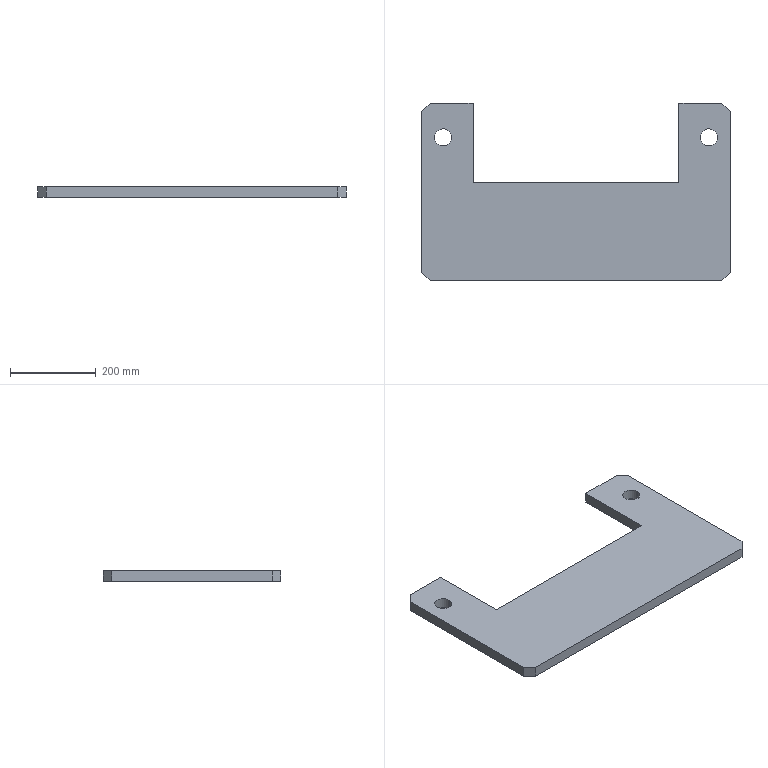Part | SolidWorks | features Chamfer 1, Extrusion 1 | 1 solid | 18 faces | box 720 x 415 x 25 mm | volume 5167168 mm3 | plane 14 | cylinder 4 | commonest cylinder face diameters 40 x4
STEP:
#1=CARTESIAN_POINT('',(650.,-80.,25.));
#2=VERTEX_POINT('',#1);
#3=CARTESIAN_POINT('',(690.,-80.,25.));
#4=VERTEX_POINT('',#3);
#5=CARTESIAN_POINT('',(670.,-80.,25.));
#6=DIRECTION('',(0.,0.,1.));
#7=DIRECTION('',(1.,0.,0.));
#8=AXIS2_PLACEMENT_3D('',#5,#6,#7);
#9=CIRCLE('',#8,20.);
#10=EDGE_CURVE('',#2,#4,#9,.T.);
#11=ORIENTED_EDGE('',*,*,#10,.T.);
#12=CARTESIAN_POINT('',(690.,-80.,0.));
#13=VERTEX_POINT('',#12);
#14=CARTESIAN_POINT('',(690.,-80.,25.));
#15=DIRECTION('',(0.,0.,-1.));
#16=VECTOR('',#15,1000.);
#17=LINE('',#14,#16);
#18=EDGE_CURVE('',#4,#13,#17,.T.);
#19=ORIENTED_EDGE('',*,*,#18,.T.);
#20=CARTESIAN_POINT('',(650.,-80.,0.));
#21=VERTEX_POINT('',#20);
#22=CARTESIAN_POINT('',(670.,-80.,0.));
#23=DIRECTION('',(0.,0.,1.));
#24=DIRECTION('',(1.,0.,0.));
#25=AXIS2_PLACEMENT_3D('',#22,#23,#24);
#26=CIRCLE('',#25,20.);
#27=EDGE_CURVE('',#21,#13,#26,.T.);
#28=ORIENTED_EDGE('',*,*,#27,.F.);
#29=CARTESIAN_POINT('',(650.,-80.,25.));
#30=DIRECTION('',(0.,0.,-1.));
#31=VECTOR('',#30,1000.);
#32=LINE('',#29,#31);
#33=EDGE_CURVE('',#2,#21,#32,.T.);
#34=ORIENTED_EDGE('',*,*,#33,.F.);
#35=EDGE_LOOP('',(#11,#19,#28,#34));
#36=FACE_OUTER_BOUND('',#35,.T.);
#37=CARTESIAN_POINT('',(670.,-80.,25.));
#38=DIRECTION('',(0.,0.,-1.));
#39=DIRECTION('',(-1.,0.,0.));
#40=AXIS2_PLACEMENT_3D('',#37,#38,#39);
#41=CYLINDRICAL_SURFACE('',#40,20.);
#42=ADVANCED_FACE('',(#36),#41,.F.);
#43=CARTESIAN_POINT('',(30.,-80.,25.));
#44=VERTEX_POINT('',#43);
#45=CARTESIAN_POINT('',(70.,-80.,25.));
#46=VERTEX_POINT('',#45);
#47=CARTESIAN_POINT('',(50.,-80.,25.));
#48=DIRECTION('',(0.,0.,1.));
#49=DIRECTION('',(1.,0.,0.));
#50=AXIS2_PLACEMENT_3D('',#47,#48,#49);
#51=CIRCLE('',#50,20.);
#52=EDGE_CURVE('',#44,#46,#51,.T.);
#53=ORIENTED_EDGE('',*,*,#52,.T.);
#54=CARTESIAN_POINT('',(70.,-80.,0.));
#55=VERTEX_POINT('',#54);
#56=CARTESIAN_POINT('',(70.,-80.,25.));
#57=DIRECTION('',(0.,0.,-1.));
#58=VECTOR('',#57,1000.);
#59=LINE('',#56,#58);
#60=EDGE_CURVE('',#46,#55,#59,.T.);
#61=ORIENTED_EDGE('',*,*,#60,.T.);
#62=CARTESIAN_POINT('',(30.,-80.,0.));
#63=VERTEX_POINT('',#62);
#64=CARTESIAN_POINT('',(50.,-80.,0.));
#65=DIRECTION('',(0.,0.,1.));
#66=DIRECTION('',(1.,0.,0.));
#67=AXIS2_PLACEMENT_3D('',#64,#65,#66);
#68=CIRCLE('',#67,20.);
#69=EDGE_CURVE('',#63,#55,#68,.T.);
#70=ORIENTED_EDGE('',*,*,#69,.F.);
#71=CARTESIAN_POINT('',(30.,-80.,25.));
#72=DIRECTION('',(0.,0.,-1.));
#73=VECTOR('',#72,1000.);
#74=LINE('',#71,#73);
#75=EDGE_CURVE('',#44,#63,#74,.T.);
#76=ORIENTED_EDGE('',*,*,#75,.F.);
#77=EDGE_LOOP('',(#53,#61,#70,#76));
#78=FACE_OUTER_BOUND('',#77,.T.);
#79=CARTESIAN_POINT('',(50.,-80.,25.));
#80=DIRECTION('',(0.,0.,-1.));
#81=DIRECTION('',(-1.,0.,0.));
#82=AXIS2_PLACEMENT_3D('',#79,#80,#81);
#83=CYLINDRICAL_SURFACE('',#82,20.);
#84=ADVANCED_FACE('',(#78),#83,.F.);
#85=CARTESIAN_POINT('',(600.,-185.,0.));
#86=VERTEX_POINT('',#85);
#87=CARTESIAN_POINT('',(120.,-185.,0.));
#88=VERTEX_POINT('',#87);
#89=CARTESIAN_POINT('',(0.,-185.,0.));
#90=DIRECTION('',(-1.,0.,0.));
#91=VECTOR('',#90,1000.);
#92=LINE('',#89,#91);
#93=EDGE_CURVE('',#86,#88,#92,.T.);
#94=ORIENTED_EDGE('',*,*,#93,.T.);
#95=CARTESIAN_POINT('',(120.,-185.,25.));
#96=VERTEX_POINT('',#95);
#97=CARTESIAN_POINT('',(120.,-185.,25.));
#98=DIRECTION('',(0.,0.,-1.));
#99=VECTOR('',#98,1000.);
#100=LINE('',#97,#99);
#101=EDGE_CURVE('',#96,#88,#100,.T.);
#102=ORIENTED_EDGE('',*,*,#101,.F.);
#103=CARTESIAN_POINT('',(600.,-185.,25.));
#104=VERTEX_POINT('',#103);
#105=CARTESIAN_POINT('',(0.,-185.,25.));
#106=DIRECTION('',(-1.,0.,0.));
#107=VECTOR('',#106,1000.);
#108=LINE('',#105,#107);
#109=EDGE_CURVE('',#104,#96,#108,.T.);
#110=ORIENTED_EDGE('',*,*,#109,.F.);
#111=CARTESIAN_POINT('',(600.,-185.,25.));
#112=DIRECTION('',(0.,0.,-1.));
#113=VECTOR('',#112,1000.);
#114=LINE('',#111,#113);
#115=EDGE_CURVE('',#104,#86,#114,.T.);
#116=ORIENTED_EDGE('',*,*,#115,.T.);
#117=EDGE_LOOP('',(#94,#102,#110,#116));
#118=FACE_OUTER_BOUND('',#117,.T.);
#119=CARTESIAN_POINT('',(0.,-185.,25.));
#120=DIRECTION('',(0.,-1.,0.));
#121=DIRECTION('',(1.,0.,0.));
#122=AXIS2_PLACEMENT_3D('',#119,#120,#121);
#123=PLANE('',#122);
#124=ADVANCED_FACE('',(#118),#123,.F.);
#125=CARTESIAN_POINT('',(120.,0.,0.));
#126=VERTEX_POINT('',#125);
#127=CARTESIAN_POINT('',(120.,0.,0.));
#128=DIRECTION('',(0.,1.,0.));
#129=VECTOR('',#128,1000.);
#130=LINE('',#127,#129);
#131=EDGE_CURVE('',#88,#126,#130,.T.);
#132=ORIENTED_EDGE('',*,*,#131,.T.);
#133=CARTESIAN_POINT('',(120.,0.,25.));
#134=VERTEX_POINT('',#133);
#135=CARTESIAN_POINT('',(120.,0.,25.));
#136=DIRECTION('',(0.,0.,-1.));
#137=VECTOR('',#136,1000.);
#138=LINE('',#135,#137);
#139=EDGE_CURVE('',#134,#126,#138,.T.);
#140=ORIENTED_EDGE('',*,*,#139,.F.);
#141=CARTESIAN_POINT('',(120.,0.,25.));
#142=DIRECTION('',(0.,1.,0.));
#143=VECTOR('',#142,1000.);
#144=LINE('',#141,#143);
#145=EDGE_CURVE('',#96,#134,#144,.T.);
#146=ORIENTED_EDGE('',*,*,#145,.F.);
#147=ORIENTED_EDGE('',*,*,#101,.T.);
#148=EDGE_LOOP('',(#132,#140,#146,#147));
#149=FACE_OUTER_BOUND('',#148,.T.);
#150=CARTESIAN_POINT('',(120.,0.,25.));
#151=DIRECTION('',(-1.,0.,0.));
#152=DIRECTION('',(0.,0.,1.));
#153=AXIS2_PLACEMENT_3D('',#150,#151,#152);
#154=PLANE('',#153);
#155=ADVANCED_FACE('',(#149),#154,.F.);
#156=CARTESIAN_POINT('',(20.,0.,0.));
#157=VERTEX_POINT('',#156);
#158=CARTESIAN_POINT('',(0.,0.,0.));
#159=DIRECTION('',(1.,0.,0.));
#160=VECTOR('',#159,1000.);
#161=LINE('',#158,#160);
#162=EDGE_CURVE('',#157,#126,#161,.T.);
#163=ORIENTED_EDGE('',*,*,#162,.F.);
#164=CARTESIAN_POINT('',(20.,0.,25.));
#165=VERTEX_POINT('',#164);
#166=CARTESIAN_POINT('',(20.,0.,25.));
#167=DIRECTION('',(0.,0.,1.));
#168=VECTOR('',#167,1000.);
#169=LINE('',#166,#168);
#170=EDGE_CURVE('',#157,#165,#169,.T.);
#171=ORIENTED_EDGE('',*,*,#170,.T.);
#172=CARTESIAN_POINT('',(0.,0.,25.));
#173=DIRECTION('',(1.,0.,0.));
#174=VECTOR('',#173,1000.);
#175=LINE('',#172,#174);
#176=EDGE_CURVE('',#165,#134,#175,.T.);
#177=ORIENTED_EDGE('',*,*,#176,.T.);
#178=ORIENTED_EDGE('',*,*,#139,.T.);
#179=EDGE_LOOP('',(#163,#171,#177,#178));
#180=FACE_OUTER_BOUND('',#179,.T.);
#181=CARTESIAN_POINT('',(0.,0.,25.));
#182=DIRECTION('',(0.,1.,0.));
#183=DIRECTION('',(0.,0.,1.));
#184=AXIS2_PLACEMENT_3D('',#181,#182,#183);
#185=PLANE('',#184);
#186=ADVANCED_FACE('',(#180),#185,.T.);
#187=CARTESIAN_POINT('',(0.,-20.,25.));
#188=VERTEX_POINT('',#187);
#189=CARTESIAN_POINT('',(0.,-395.,25.));
#190=VERTEX_POINT('',#189);
#191=CARTESIAN_POINT('',(0.,0.,25.));
#192=DIRECTION('',(0.,-1.,0.));
#193=VECTOR('',#192,1000.);
#194=LINE('',#191,#193);
#195=EDGE_CURVE('',#188,#190,#194,.T.);
#196=ORIENTED_EDGE('',*,*,#195,.F.);
#197=CARTESIAN_POINT('',(0.,-20.,0.));
#198=VERTEX_POINT('',#197);
#199=CARTESIAN_POINT('',(0.,-20.,0.));
#200=DIRECTION('',(0.,0.,-1.));
#201=VECTOR('',#200,1000.);
#202=LINE('',#199,#201);
#203=EDGE_CURVE('',#188,#198,#202,.T.);
#204=ORIENTED_EDGE('',*,*,#203,.T.);
#205=CARTESIAN_POINT('',(0.,-395.,0.));
#206=VERTEX_POINT('',#205);
#207=CARTESIAN_POINT('',(0.,0.,0.));
#208=DIRECTION('',(0.,-1.,0.));
#209=VECTOR('',#208,1000.);
#210=LINE('',#207,#209);
#211=EDGE_CURVE('',#198,#206,#210,.T.);
#212=ORIENTED_EDGE('',*,*,#211,.T.);
#213=CARTESIAN_POINT('',(0.,-395.,25.));
#214=DIRECTION('',(0.,0.,1.));
#215=VECTOR('',#214,1000.);
#216=LINE('',#213,#215);
#217=EDGE_CURVE('',#206,#190,#216,.T.);
#218=ORIENTED_EDGE('',*,*,#217,.T.);
#219=EDGE_LOOP('',(#196,#204,#212,#218));
#220=FACE_OUTER_BOUND('',#219,.T.);
#221=CARTESIAN_POINT('',(0.,0.,25.));
#222=DIRECTION('',(1.,0.,0.));
#223=DIRECTION('',(0.,1.,0.));
#224=AXIS2_PLACEMENT_3D('',#221,#222,#223);
#225=PLANE('',#224);
#226=ADVANCED_FACE('',(#220),#225,.F.);
#227=CARTESIAN_POINT('',(20.,-415.,25.));
#228=VERTEX_POINT('',#227);
#229=CARTESIAN_POINT('',(700.,-415.,25.));
#230=VERTEX_POINT('',#229);
#231=CARTESIAN_POINT('',(0.,-415.,25.));
#232=DIRECTION('',(1.,0.,0.));
#233=VECTOR('',#232,1000.);
#234=LINE('',#231,#233);
#235=EDGE_CURVE('',#228,#230,#234,.T.);
#236=ORIENTED_EDGE('',*,*,#235,.F.);
#237=CARTESIAN_POINT('',(20.,-415.,0.));
#238=VERTEX_POINT('',#237);
#239=CARTESIAN_POINT('',(20.,-415.,25.));
#240=DIRECTION('',(0.,0.,-1.));
#241=VECTOR('',#240,1000.);
#242=LINE('',#239,#241);
#243=EDGE_CURVE('',#228,#238,#242,.T.);
#244=ORIENTED_EDGE('',*,*,#243,.T.);
#245=CARTESIAN_POINT('',(700.,-415.,0.));
#246=VERTEX_POINT('',#245);
#247=CARTESIAN_POINT('',(0.,-415.,0.));
#248=DIRECTION('',(1.,0.,0.));
#249=VECTOR('',#248,1000.);
#250=LINE('',#247,#249);
#251=EDGE_CURVE('',#238,#246,#250,.T.);
#252=ORIENTED_EDGE('',*,*,#251,.T.);
#253=CARTESIAN_POINT('',(700.,-415.,25.));
#254=DIRECTION('',(0.,0.,1.));
#255=VECTOR('',#254,1000.);
#256=LINE('',#253,#255);
#257=EDGE_CURVE('',#246,#230,#256,.T.);
#258=ORIENTED_EDGE('',*,*,#257,.T.);
#259=EDGE_LOOP('',(#236,#244,#252,#258));
#260=FACE_OUTER_BOUND('',#259,.T.);
#261=CARTESIAN_POINT('',(0.,-415.,25.));
#262=DIRECTION('',(0.,1.,0.));
#263=DIRECTION('',(0.,0.,1.));
#264=AXIS2_PLACEMENT_3D('',#261,#262,#263);
#265=PLANE('',#264);
#266=ADVANCED_FACE('',(#260),#265,.F.);
#267=CARTESIAN_POINT('',(720.,-20.,25.));
#268=VERTEX_POINT('',#267);
#269=CARTESIAN_POINT('',(720.,-395.,25.));
#270=VERTEX_POINT('',#269);
#271=CARTESIAN_POINT('',(720.,0.,25.));
#272=DIRECTION('',(0.,-1.,0.));
#273=VECTOR('',#272,1000.);
#274=LINE('',#271,#273);
#275=EDGE_CURVE('',#268,#270,#274,.T.);
#276=ORIENTED_EDGE('',*,*,#275,.T.);
#277=CARTESIAN_POINT('',(720.,-395.,0.));
#278=VERTEX_POINT('',#277);
#279=CARTESIAN_POINT('',(720.,-395.,0.));
#280=DIRECTION('',(0.,0.,-1.));
#281=VECTOR('',#280,1000.);
#282=LINE('',#279,#281);
#283=EDGE_CURVE('',#270,#278,#282,.T.);
#284=ORIENTED_EDGE('',*,*,#283,.T.);
#285=CARTESIAN_POINT('',(720.,-20.,0.));
#286=VERTEX_POINT('',#285);
#287=CARTESIAN_POINT('',(720.,0.,0.));
#288=DIRECTION('',(0.,-1.,0.));
#289=VECTOR('',#288,1000.);
#290=LINE('',#287,#289);
#291=EDGE_CURVE('',#286,#278,#290,.T.);
#292=ORIENTED_EDGE('',*,*,#291,.F.);
#293=CARTESIAN_POINT('',(720.,-20.,25.));
#294=DIRECTION('',(0.,0.,1.));
#295=VECTOR('',#294,1000.);
#296=LINE('',#293,#295);
#297=EDGE_CURVE('',#286,#268,#296,.T.);
#298=ORIENTED_EDGE('',*,*,#297,.T.);
#299=EDGE_LOOP('',(#276,#284,#292,#298));
#300=FACE_OUTER_BOUND('',#299,.T.);
#301=CARTESIAN_POINT('',(720.,0.,25.));
#302=DIRECTION('',(1.,0.,0.));
#303=DIRECTION('',(0.,1.,0.));
#304=AXIS2_PLACEMENT_3D('',#301,#302,#303);
#305=PLANE('',#304);
#306=ADVANCED_FACE('',(#300),#305,.T.);
#307=CARTESIAN_POINT('',(600.,0.,25.));
#308=VERTEX_POINT('',#307);
#309=CARTESIAN_POINT('',(700.,0.,25.));
#310=VERTEX_POINT('',#309);
#311=CARTESIAN_POINT('',(0.,0.,25.));
#312=DIRECTION('',(1.,0.,0.));
#313=VECTOR('',#312,1000.);
#314=LINE('',#311,#313);
#315=EDGE_CURVE('',#308,#310,#314,.T.);
#316=ORIENTED_EDGE('',*,*,#315,.T.);
#317=CARTESIAN_POINT('',(700.,0.,0.));
#318=VERTEX_POINT('',#317);
#319=CARTESIAN_POINT('',(700.,0.,25.));
#320=DIRECTION('',(0.,0.,-1.));
#321=VECTOR('',#320,1000.);
#322=LINE('',#319,#321);
#323=EDGE_CURVE('',#310,#318,#322,.T.);
#324=ORIENTED_EDGE('',*,*,#323,.T.);
#325=CARTESIAN_POINT('',(600.,0.,0.));
#326=VERTEX_POINT('',#325);
#327=CARTESIAN_POINT('',(0.,0.,0.));
#328=DIRECTION('',(1.,0.,0.));
#329=VECTOR('',#328,1000.);
#330=LINE('',#327,#329);
#331=EDGE_CURVE('',#326,#318,#330,.T.);
#332=ORIENTED_EDGE('',*,*,#331,.F.);
#333=CARTESIAN_POINT('',(600.,0.,25.));
#334=DIRECTION('',(0.,0.,-1.));
#335=VECTOR('',#334,1000.);
#336=LINE('',#333,#335);
#337=EDGE_CURVE('',#308,#326,#336,.T.);
#338=ORIENTED_EDGE('',*,*,#337,.F.);
#339=EDGE_LOOP('',(#316,#324,#332,#338));
#340=FACE_OUTER_BOUND('',#339,.T.);
#341=CARTESIAN_POINT('',(0.,0.,25.));
#342=DIRECTION('',(0.,1.,0.));
#343=DIRECTION('',(0.,0.,1.));
#344=AXIS2_PLACEMENT_3D('',#341,#342,#343);
#345=PLANE('',#344);
#346=ADVANCED_FACE('',(#340),#345,.T.);
#347=ORIENTED_EDGE('',*,*,#60,.F.);
#348=CARTESIAN_POINT('',(50.,-80.,25.));
#349=DIRECTION('',(0.,0.,1.));
#350=DIRECTION('',(1.,0.,0.));
#351=AXIS2_PLACEMENT_3D('',#348,#349,#350);
#352=CIRCLE('',#351,20.);
#353=EDGE_CURVE('',#46,#44,#352,.T.);
#354=ORIENTED_EDGE('',*,*,#353,.T.);
#355=ORIENTED_EDGE('',*,*,#75,.T.);
#356=CARTESIAN_POINT('',(50.,-80.,0.));
#357=DIRECTION('',(0.,0.,1.));
#358=DIRECTION('',(1.,0.,0.));
#359=AXIS2_PLACEMENT_3D('',#356,#357,#358);
#360=CIRCLE('',#359,20.);
#361=EDGE_CURVE('',#55,#63,#360,.T.);
#362=ORIENTED_EDGE('',*,*,#361,.F.);
#363=EDGE_LOOP('',(#347,#354,#355,#362));
#364=FACE_OUTER_BOUND('',#363,.T.);
#365=CARTESIAN_POINT('',(50.,-80.,25.));
#366=DIRECTION('',(0.,0.,-1.));
#367=DIRECTION('',(-1.,0.,0.));
#368=AXIS2_PLACEMENT_3D('',#365,#366,#367);
#369=CYLINDRICAL_SURFACE('',#368,20.);
#370=ADVANCED_FACE('',(#364),#369,.F.);
#371=ORIENTED_EDGE('',*,*,#18,.F.);
#372=CARTESIAN_POINT('',(670.,-80.,25.));
#373=DIRECTION('',(0.,0.,1.));
#374=DIRECTION('',(1.,0.,0.));
#375=AXIS2_PLACEMENT_3D('',#372,#373,#374);
#376=CIRCLE('',#375,20.);
#377=EDGE_CURVE('',#4,#2,#376,.T.);
#378=ORIENTED_EDGE('',*,*,#377,.T.);
#379=ORIENTED_EDGE('',*,*,#33,.T.);
#380=CARTESIAN_POINT('',(670.,-80.,0.));
#381=DIRECTION('',(0.,0.,1.));
#382=DIRECTION('',(1.,0.,0.));
#383=AXIS2_PLACEMENT_3D('',#380,#381,#382);
#384=CIRCLE('',#383,20.);
#385=EDGE_CURVE('',#13,#21,#384,.T.);
#386=ORIENTED_EDGE('',*,*,#385,.F.);
#387=EDGE_LOOP('',(#371,#378,#379,#386));
#388=FACE_OUTER_BOUND('',#387,.T.);
#389=CARTESIAN_POINT('',(670.,-80.,25.));
#390=DIRECTION('',(0.,0.,-1.));
#391=DIRECTION('',(-1.,0.,0.));
#392=AXIS2_PLACEMENT_3D('',#389,#390,#391);
#393=CYLINDRICAL_SURFACE('',#392,20.);
#394=ADVANCED_FACE('',(#388),#393,.F.);
#395=CARTESIAN_POINT('',(600.,0.,0.));
#396=DIRECTION('',(0.,1.,0.));
#397=VECTOR('',#396,1000.);
#398=LINE('',#395,#397);
#399=EDGE_CURVE('',#86,#326,#398,.T.);
#400=ORIENTED_EDGE('',*,*,#399,.F.);
#401=ORIENTED_EDGE('',*,*,#115,.F.);
#402=CARTESIAN_POINT('',(600.,0.,25.));
#403=DIRECTION('',(0.,1.,0.));
#404=VECTOR('',#403,1000.);
#405=LINE('',#402,#404);
#406=EDGE_CURVE('',#104,#308,#405,.T.);
#407=ORIENTED_EDGE('',*,*,#406,.T.);
#408=ORIENTED_EDGE('',*,*,#337,.T.);
#409=EDGE_LOOP('',(#400,#401,#407,#408));
#410=FACE_OUTER_BOUND('',#409,.T.);
#411=CARTESIAN_POINT('',(600.,0.,25.));
#412=DIRECTION('',(-1.,0.,0.));
#413=DIRECTION('',(0.,0.,1.));
#414=AXIS2_PLACEMENT_3D('',#411,#412,#413);
#415=PLANE('',#414);
#416=ADVANCED_FACE('',(#410),#415,.T.);
#417=ORIENTED_EDGE('',*,*,#10,.F.);
#418=ORIENTED_EDGE('',*,*,#377,.F.);
#419=EDGE_LOOP('',(#417,#418));
#420=FACE_BOUND('',#419,.T.);
#421=ORIENTED_EDGE('',*,*,#52,.F.);
#422=ORIENTED_EDGE('',*,*,#353,.F.);
#423=EDGE_LOOP('',(#421,#422));
#424=FACE_BOUND('',#423,.T.);
#425=ORIENTED_EDGE('',*,*,#176,.F.);
#426=CARTESIAN_POINT('',(10.,-10.,25.));
#427=DIRECTION('',(-0.7071,-0.7071,0.));
#428=VECTOR('',#427,1000.);
#429=LINE('',#426,#428);
#430=EDGE_CURVE('',#165,#188,#429,.T.);
#431=ORIENTED_EDGE('',*,*,#430,.T.);
#432=ORIENTED_EDGE('',*,*,#195,.T.);
#433=CARTESIAN_POINT('',(-197.5,-197.5,25.));
#434=DIRECTION('',(0.7071,-0.7071,0.));
#435=VECTOR('',#434,1000.);
#436=LINE('',#433,#435);
#437=EDGE_CURVE('',#190,#228,#436,.T.);
#438=ORIENTED_EDGE('',*,*,#437,.T.);
#439=ORIENTED_EDGE('',*,*,#235,.T.);
#440=CARTESIAN_POINT('',(557.5,-557.5,25.));
#441=DIRECTION('',(0.7071,0.7071,0.));
#442=VECTOR('',#441,1000.);
#443=LINE('',#440,#442);
#444=EDGE_CURVE('',#230,#270,#443,.T.);
#445=ORIENTED_EDGE('',*,*,#444,.T.);
#446=ORIENTED_EDGE('',*,*,#275,.F.);
#447=CARTESIAN_POINT('',(350.,350.,25.));
#448=DIRECTION('',(-0.7071,0.7071,0.));
#449=VECTOR('',#448,1000.);
#450=LINE('',#447,#449);
#451=EDGE_CURVE('',#268,#310,#450,.T.);
#452=ORIENTED_EDGE('',*,*,#451,.T.);
#453=ORIENTED_EDGE('',*,*,#315,.F.);
#454=ORIENTED_EDGE('',*,*,#406,.F.);
#455=ORIENTED_EDGE('',*,*,#109,.T.);
#456=ORIENTED_EDGE('',*,*,#145,.T.);
#457=EDGE_LOOP('',(#425,#431,#432,#438,#439,#445,#446,#452,#453,#454,#455,#456));
#458=FACE_OUTER_BOUND('',#457,.T.);
#459=CARTESIAN_POINT('',(0.,0.,25.));
#460=DIRECTION('',(0.,0.,1.));
#461=DIRECTION('',(1.,0.,0.));
#462=AXIS2_PLACEMENT_3D('',#459,#460,#461);
#463=PLANE('',#462);
#464=ADVANCED_FACE('',(#420,#424,#458),#463,.T.);
#465=ORIENTED_EDGE('',*,*,#27,.T.);
#466=ORIENTED_EDGE('',*,*,#385,.T.);
#467=EDGE_LOOP('',(#465,#466));
#468=FACE_BOUND('',#467,.T.);
#469=ORIENTED_EDGE('',*,*,#69,.T.);
#470=ORIENTED_EDGE('',*,*,#361,.T.);
#471=EDGE_LOOP('',(#469,#470));
#472=FACE_BOUND('',#471,.T.);
#473=ORIENTED_EDGE('',*,*,#211,.F.);
#474=CARTESIAN_POINT('',(0.,-20.,0.));
#475=DIRECTION('',(0.7071,0.7071,0.));
#476=VECTOR('',#475,1000.);
#477=LINE('',#474,#476);
#478=EDGE_CURVE('',#198,#157,#477,.T.);
#479=ORIENTED_EDGE('',*,*,#478,.T.);
#480=ORIENTED_EDGE('',*,*,#162,.T.);
#481=ORIENTED_EDGE('',*,*,#131,.F.);
#482=ORIENTED_EDGE('',*,*,#93,.F.);
#483=ORIENTED_EDGE('',*,*,#399,.T.);
#484=ORIENTED_EDGE('',*,*,#331,.T.);
#485=CARTESIAN_POINT('',(700.,0.,0.));
#486=DIRECTION('',(0.7071,-0.7071,0.));
#487=VECTOR('',#486,1000.);
#488=LINE('',#485,#487);
#489=EDGE_CURVE('',#318,#286,#488,.T.);
#490=ORIENTED_EDGE('',*,*,#489,.T.);
#491=ORIENTED_EDGE('',*,*,#291,.T.);
#492=CARTESIAN_POINT('',(720.,-395.,0.));
#493=DIRECTION('',(-0.7071,-0.7071,0.));
#494=VECTOR('',#493,1000.);
#495=LINE('',#492,#494);
#496=EDGE_CURVE('',#278,#246,#495,.T.);
#497=ORIENTED_EDGE('',*,*,#496,.T.);
#498=ORIENTED_EDGE('',*,*,#251,.F.);
#499=CARTESIAN_POINT('',(20.,-415.,0.));
#500=DIRECTION('',(-0.7071,0.7071,0.));
#501=VECTOR('',#500,1000.);
#502=LINE('',#499,#501);
#503=EDGE_CURVE('',#238,#206,#502,.T.);
#504=ORIENTED_EDGE('',*,*,#503,.T.);
#505=EDGE_LOOP('',(#473,#479,#480,#481,#482,#483,#484,#490,#491,#497,#498,#504));
#506=FACE_OUTER_BOUND('',#505,.T.);
#507=CARTESIAN_POINT('',(0.,0.,0.));
#508=DIRECTION('',(0.,0.,1.));
#509=DIRECTION('',(1.,0.,0.));
#510=AXIS2_PLACEMENT_3D('',#507,#508,#509);
#511=PLANE('',#510);
#512=ADVANCED_FACE('',(#468,#472,#506),#511,.F.);
#513=ORIENTED_EDGE('',*,*,#430,.F.);
#514=ORIENTED_EDGE('',*,*,#170,.F.);
#515=ORIENTED_EDGE('',*,*,#478,.F.);
#516=ORIENTED_EDGE('',*,*,#203,.F.);
#517=EDGE_LOOP('',(#513,#514,#515,#516));
#518=FACE_OUTER_BOUND('',#517,.T.);
#519=CARTESIAN_POINT('',(0.,-20.,25.));
#520=DIRECTION('',(-0.7071,0.7071,0.));
#521=DIRECTION('',(0.,0.,1.));
#522=AXIS2_PLACEMENT_3D('',#519,#520,#521);
#523=PLANE('',#522);
#524=ADVANCED_FACE('',(#518),#523,.T.);
#525=ORIENTED_EDGE('',*,*,#437,.F.);
#526=ORIENTED_EDGE('',*,*,#217,.F.);
#527=ORIENTED_EDGE('',*,*,#503,.F.);
#528=ORIENTED_EDGE('',*,*,#243,.F.);
#529=EDGE_LOOP('',(#525,#526,#527,#528));
#530=FACE_OUTER_BOUND('',#529,.T.);
#531=CARTESIAN_POINT('',(20.,-415.,25.));
#532=DIRECTION('',(0.7071,0.7071,0.));
#533=DIRECTION('',(0.,0.,-1.));
#534=AXIS2_PLACEMENT_3D('',#531,#532,#533);
#535=PLANE('',#534);
#536=ADVANCED_FACE('',(#530),#535,.F.);
#537=ORIENTED_EDGE('',*,*,#444,.F.);
#538=ORIENTED_EDGE('',*,*,#257,.F.);
#539=ORIENTED_EDGE('',*,*,#496,.F.);
#540=ORIENTED_EDGE('',*,*,#283,.F.);
#541=EDGE_LOOP('',(#537,#538,#539,#540));
#542=FACE_OUTER_BOUND('',#541,.T.);
#543=CARTESIAN_POINT('',(720.,-395.,25.));
#544=DIRECTION('',(0.7071,-0.7071,0.));
#545=DIRECTION('',(0.,0.,1.));
#546=AXIS2_PLACEMENT_3D('',#543,#544,#545);
#547=PLANE('',#546);
#548=ADVANCED_FACE('',(#542),#547,.T.);
#549=ORIENTED_EDGE('',*,*,#451,.F.);
#550=ORIENTED_EDGE('',*,*,#297,.F.);
#551=ORIENTED_EDGE('',*,*,#489,.F.);
#552=ORIENTED_EDGE('',*,*,#323,.F.);
#553=EDGE_LOOP('',(#549,#550,#551,#552));
#554=FACE_OUTER_BOUND('',#553,.T.);
#555=CARTESIAN_POINT('',(700.,0.,25.));
#556=DIRECTION('',(-0.7071,-0.7071,0.));
#557=DIRECTION('',(0.,0.,-1.));
#558=AXIS2_PLACEMENT_3D('',#555,#556,#557);
#559=PLANE('',#558);
#560=ADVANCED_FACE('',(#554),#559,.F.);
#561=CLOSED_SHELL('',(#42,#84,#124,#155,#186,#226,#266,#306,#346,#370,#394,#416,#464,#512,#524,#536,#548,#560));
#562=MANIFOLD_SOLID_BREP('',#561);
#563=CARTESIAN_POINT('',(0.,0.,0.));
#564=DIRECTION('',(0.,0.,1.));
#565=DIRECTION('',(1.,0.,0.));
#566=AXIS2_PLACEMENT_3D('',#563,#564,#565);
#567=(LENGTH_UNIT()NAMED_UNIT(*)SI_UNIT(.MILLI.,.METRE.));
#568=UNCERTAINTY_MEASURE_WITH_UNIT(LENGTH_MEASURE(0.00001),#567,'','');
#569=(NAMED_UNIT(*)PLANE_ANGLE_UNIT()SI_UNIT($,.RADIAN.));
#570=(NAMED_UNIT(*)SI_UNIT($,.STERADIAN.)SOLID_ANGLE_UNIT());
#571=(GEOMETRIC_REPRESENTATION_CONTEXT(3)GLOBAL_UNCERTAINTY_ASSIGNED_CONTEXT((#568))GLOBAL_UNIT_ASSIGNED_CONTEXT((#567,#569,#570))REPRESENTATION_CONTEXT('',''));
#572=ADVANCED_BREP_SHAPE_REPRESENTATION('',(#562,#566),#571);